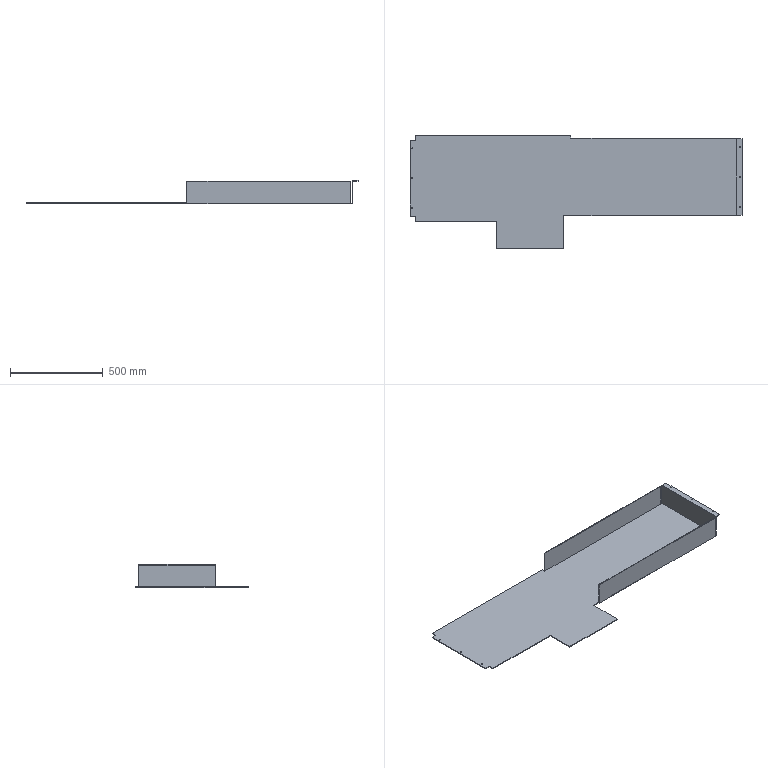Part | STEP file | Guard 8 | 1 solid | 44 faces | box 1787 x 612 x 124 mm | volume 4313397 mm3 | plane 32 | cylinder 12 | commonest cylinder face diameters 6 x12
STEP:
#1=CARTESIAN_POINT('',(16.,199.5,4.));
#2=VERTEX_POINT('',#1);
#3=CARTESIAN_POINT('',(10.,199.5,4.));
#4=VERTEX_POINT('',#3);
#5=CARTESIAN_POINT('',(13.,199.5,4.));
#6=DIRECTION('',(0.,0.,-1.));
#7=DIRECTION('',(-1.,0.,0.));
#8=AXIS2_PLACEMENT_3D('',#5,#6,#7);
#9=CIRCLE('',#8,3.);
#10=EDGE_CURVE('',#2,#4,#9,.T.);
#11=ORIENTED_EDGE('',*,*,#10,.F.);
#12=CARTESIAN_POINT('',(16.,199.5,0.));
#13=VERTEX_POINT('',#12);
#14=CARTESIAN_POINT('',(16.,199.5,10.));
#15=DIRECTION('',(0.,0.,-1.));
#16=VECTOR('',#15,1000.);
#17=LINE('',#14,#16);
#18=EDGE_CURVE('',#2,#13,#17,.T.);
#19=ORIENTED_EDGE('',*,*,#18,.T.);
#20=CARTESIAN_POINT('',(10.,199.5,0.));
#21=VERTEX_POINT('',#20);
#22=CARTESIAN_POINT('',(13.,199.5,0.));
#23=DIRECTION('',(0.,0.,-1.));
#24=DIRECTION('',(-1.,0.,0.));
#25=AXIS2_PLACEMENT_3D('',#22,#23,#24);
#26=CIRCLE('',#25,3.);
#27=EDGE_CURVE('',#13,#21,#26,.T.);
#28=ORIENTED_EDGE('',*,*,#27,.T.);
#29=CARTESIAN_POINT('',(10.,199.5,10.));
#30=DIRECTION('',(0.,0.,-1.));
#31=VECTOR('',#30,1000.);
#32=LINE('',#29,#31);
#33=EDGE_CURVE('',#4,#21,#32,.T.);
#34=ORIENTED_EDGE('',*,*,#33,.F.);
#35=EDGE_LOOP('',(#11,#19,#28,#34));
#36=FACE_OUTER_BOUND('',#35,.T.);
#37=CARTESIAN_POINT('',(13.,199.5,10.));
#38=DIRECTION('',(0.,0.,-1.));
#39=DIRECTION('',(-1.,0.,0.));
#40=AXIS2_PLACEMENT_3D('',#37,#38,#39);
#41=CYLINDRICAL_SURFACE('',#40,3.);
#42=ADVANCED_FACE('',(#36),#41,.F.);
#43=CARTESIAN_POINT('',(16.,39.5,4.));
#44=VERTEX_POINT('',#43);
#45=CARTESIAN_POINT('',(10.,39.5,4.));
#46=VERTEX_POINT('',#45);
#47=CARTESIAN_POINT('',(13.,39.5,4.));
#48=DIRECTION('',(0.,0.,-1.));
#49=DIRECTION('',(-1.,0.,0.));
#50=AXIS2_PLACEMENT_3D('',#47,#48,#49);
#51=CIRCLE('',#50,3.);
#52=EDGE_CURVE('',#44,#46,#51,.T.);
#53=ORIENTED_EDGE('',*,*,#52,.F.);
#54=CARTESIAN_POINT('',(16.,39.5,0.));
#55=VERTEX_POINT('',#54);
#56=CARTESIAN_POINT('',(16.,39.5,10.));
#57=DIRECTION('',(0.,0.,-1.));
#58=VECTOR('',#57,1000.);
#59=LINE('',#56,#58);
#60=EDGE_CURVE('',#44,#55,#59,.T.);
#61=ORIENTED_EDGE('',*,*,#60,.T.);
#62=CARTESIAN_POINT('',(10.,39.5,0.));
#63=VERTEX_POINT('',#62);
#64=CARTESIAN_POINT('',(13.,39.5,0.));
#65=DIRECTION('',(0.,0.,-1.));
#66=DIRECTION('',(-1.,0.,0.));
#67=AXIS2_PLACEMENT_3D('',#64,#65,#66);
#68=CIRCLE('',#67,3.);
#69=EDGE_CURVE('',#55,#63,#68,.T.);
#70=ORIENTED_EDGE('',*,*,#69,.T.);
#71=CARTESIAN_POINT('',(10.,39.5,10.));
#72=DIRECTION('',(0.,0.,-1.));
#73=VECTOR('',#72,1000.);
#74=LINE('',#71,#73);
#75=EDGE_CURVE('',#46,#63,#74,.T.);
#76=ORIENTED_EDGE('',*,*,#75,.F.);
#77=EDGE_LOOP('',(#53,#61,#70,#76));
#78=FACE_OUTER_BOUND('',#77,.T.);
#79=CARTESIAN_POINT('',(13.,39.5,10.));
#80=DIRECTION('',(0.,0.,-1.));
#81=DIRECTION('',(-1.,0.,0.));
#82=AXIS2_PLACEMENT_3D('',#79,#80,#81);
#83=CYLINDRICAL_SURFACE('',#82,3.);
#84=ADVANCED_FACE('',(#78),#83,.F.);
#85=CARTESIAN_POINT('',(16.,359.5,4.));
#86=VERTEX_POINT('',#85);
#87=CARTESIAN_POINT('',(10.,359.5,4.));
#88=VERTEX_POINT('',#87);
#89=CARTESIAN_POINT('',(13.,359.5,4.));
#90=DIRECTION('',(0.,0.,-1.));
#91=DIRECTION('',(-1.,0.,0.));
#92=AXIS2_PLACEMENT_3D('',#89,#90,#91);
#93=CIRCLE('',#92,3.);
#94=EDGE_CURVE('',#86,#88,#93,.T.);
#95=ORIENTED_EDGE('',*,*,#94,.F.);
#96=CARTESIAN_POINT('',(16.,359.5,0.));
#97=VERTEX_POINT('',#96);
#98=CARTESIAN_POINT('',(16.,359.5,10.));
#99=DIRECTION('',(0.,0.,-1.));
#100=VECTOR('',#99,1000.);
#101=LINE('',#98,#100);
#102=EDGE_CURVE('',#86,#97,#101,.T.);
#103=ORIENTED_EDGE('',*,*,#102,.T.);
#104=CARTESIAN_POINT('',(10.,359.5,0.));
#105=VERTEX_POINT('',#104);
#106=CARTESIAN_POINT('',(13.,359.5,0.));
#107=DIRECTION('',(0.,0.,-1.));
#108=DIRECTION('',(-1.,0.,0.));
#109=AXIS2_PLACEMENT_3D('',#106,#107,#108);
#110=CIRCLE('',#109,3.);
#111=EDGE_CURVE('',#97,#105,#110,.T.);
#112=ORIENTED_EDGE('',*,*,#111,.T.);
#113=CARTESIAN_POINT('',(10.,359.5,10.));
#114=DIRECTION('',(0.,0.,-1.));
#115=VECTOR('',#114,1000.);
#116=LINE('',#113,#115);
#117=EDGE_CURVE('',#88,#105,#116,.T.);
#118=ORIENTED_EDGE('',*,*,#117,.F.);
#119=EDGE_LOOP('',(#95,#103,#112,#118));
#120=FACE_OUTER_BOUND('',#119,.T.);
#121=CARTESIAN_POINT('',(13.,359.5,10.));
#122=DIRECTION('',(0.,0.,-1.));
#123=DIRECTION('',(-1.,0.,0.));
#124=AXIS2_PLACEMENT_3D('',#121,#122,#123);
#125=CYLINDRICAL_SURFACE('',#124,3.);
#126=ADVANCED_FACE('',(#120),#125,.F.);
#127=CARTESIAN_POINT('',(1774.,205.5,124.));
#128=VERTEX_POINT('',#127);
#129=CARTESIAN_POINT('',(1780.,205.5,124.));
#130=VERTEX_POINT('',#129);
#131=CARTESIAN_POINT('',(1777.,205.5,124.));
#132=DIRECTION('',(0.,0.,1.));
#133=DIRECTION('',(1.,0.,0.));
#134=AXIS2_PLACEMENT_3D('',#131,#132,#133);
#135=CIRCLE('',#134,3.);
#136=EDGE_CURVE('',#128,#130,#135,.T.);
#137=ORIENTED_EDGE('',*,*,#136,.T.);
#138=CARTESIAN_POINT('',(1780.,205.5,121.));
#139=VERTEX_POINT('',#138);
#140=CARTESIAN_POINT('',(1780.,205.5,131.));
#141=DIRECTION('',(0.,0.,-1.));
#142=VECTOR('',#141,1000.);
#143=LINE('',#140,#142);
#144=EDGE_CURVE('',#130,#139,#143,.T.);
#145=ORIENTED_EDGE('',*,*,#144,.T.);
#146=CARTESIAN_POINT('',(1774.,205.5,121.));
#147=VERTEX_POINT('',#146);
#148=CARTESIAN_POINT('',(1777.,205.5,121.));
#149=DIRECTION('',(0.,0.,-1.));
#150=DIRECTION('',(-1.,0.,0.));
#151=AXIS2_PLACEMENT_3D('',#148,#149,#150);
#152=CIRCLE('',#151,3.);
#153=EDGE_CURVE('',#139,#147,#152,.T.);
#154=ORIENTED_EDGE('',*,*,#153,.T.);
#155=CARTESIAN_POINT('',(1774.,205.5,131.));
#156=DIRECTION('',(0.,0.,-1.));
#157=VECTOR('',#156,1000.);
#158=LINE('',#155,#157);
#159=EDGE_CURVE('',#128,#147,#158,.T.);
#160=ORIENTED_EDGE('',*,*,#159,.F.);
#161=EDGE_LOOP('',(#137,#145,#154,#160));
#162=FACE_OUTER_BOUND('',#161,.T.);
#163=CARTESIAN_POINT('',(1777.,205.5,131.));
#164=DIRECTION('',(0.,0.,-1.));
#165=DIRECTION('',(-1.,0.,0.));
#166=AXIS2_PLACEMENT_3D('',#163,#164,#165);
#167=CYLINDRICAL_SURFACE('',#166,3.);
#168=ADVANCED_FACE('',(#162),#167,.F.);
#169=CARTESIAN_POINT('',(1774.,45.5,124.));
#170=VERTEX_POINT('',#169);
#171=CARTESIAN_POINT('',(1780.,45.5,124.));
#172=VERTEX_POINT('',#171);
#173=CARTESIAN_POINT('',(1777.,45.5,124.));
#174=DIRECTION('',(0.,0.,1.));
#175=DIRECTION('',(1.,0.,0.));
#176=AXIS2_PLACEMENT_3D('',#173,#174,#175);
#177=CIRCLE('',#176,3.);
#178=EDGE_CURVE('',#170,#172,#177,.T.);
#179=ORIENTED_EDGE('',*,*,#178,.T.);
#180=CARTESIAN_POINT('',(1780.,45.5,121.));
#181=VERTEX_POINT('',#180);
#182=CARTESIAN_POINT('',(1780.,45.5,131.));
#183=DIRECTION('',(0.,0.,-1.));
#184=VECTOR('',#183,1000.);
#185=LINE('',#182,#184);
#186=EDGE_CURVE('',#172,#181,#185,.T.);
#187=ORIENTED_EDGE('',*,*,#186,.T.);
#188=CARTESIAN_POINT('',(1774.,45.5,121.));
#189=VERTEX_POINT('',#188);
#190=CARTESIAN_POINT('',(1777.,45.5,121.));
#191=DIRECTION('',(0.,0.,-1.));
#192=DIRECTION('',(-1.,0.,0.));
#193=AXIS2_PLACEMENT_3D('',#190,#191,#192);
#194=CIRCLE('',#193,3.);
#195=EDGE_CURVE('',#181,#189,#194,.T.);
#196=ORIENTED_EDGE('',*,*,#195,.T.);
#197=CARTESIAN_POINT('',(1774.,45.5,131.));
#198=DIRECTION('',(0.,0.,-1.));
#199=VECTOR('',#198,1000.);
#200=LINE('',#197,#199);
#201=EDGE_CURVE('',#170,#189,#200,.T.);
#202=ORIENTED_EDGE('',*,*,#201,.F.);
#203=EDGE_LOOP('',(#179,#187,#196,#202));
#204=FACE_OUTER_BOUND('',#203,.T.);
#205=CARTESIAN_POINT('',(1777.,45.5,131.));
#206=DIRECTION('',(0.,0.,-1.));
#207=DIRECTION('',(-1.,0.,0.));
#208=AXIS2_PLACEMENT_3D('',#205,#206,#207);
#209=CYLINDRICAL_SURFACE('',#208,3.);
#210=ADVANCED_FACE('',(#204),#209,.F.);
#211=CARTESIAN_POINT('',(1774.,365.5,124.));
#212=VERTEX_POINT('',#211);
#213=CARTESIAN_POINT('',(1780.,365.5,124.));
#214=VERTEX_POINT('',#213);
#215=CARTESIAN_POINT('',(1777.,365.5,124.));
#216=DIRECTION('',(0.,0.,1.));
#217=DIRECTION('',(1.,0.,0.));
#218=AXIS2_PLACEMENT_3D('',#215,#216,#217);
#219=CIRCLE('',#218,3.);
#220=EDGE_CURVE('',#212,#214,#219,.T.);
#221=ORIENTED_EDGE('',*,*,#220,.T.);
#222=CARTESIAN_POINT('',(1780.,365.5,121.));
#223=VERTEX_POINT('',#222);
#224=CARTESIAN_POINT('',(1780.,365.5,131.));
#225=DIRECTION('',(0.,0.,-1.));
#226=VECTOR('',#225,1000.);
#227=LINE('',#224,#226);
#228=EDGE_CURVE('',#214,#223,#227,.T.);
#229=ORIENTED_EDGE('',*,*,#228,.T.);
#230=CARTESIAN_POINT('',(1774.,365.5,121.));
#231=VERTEX_POINT('',#230);
#232=CARTESIAN_POINT('',(1777.,365.5,121.));
#233=DIRECTION('',(0.,0.,-1.));
#234=DIRECTION('',(-1.,0.,0.));
#235=AXIS2_PLACEMENT_3D('',#232,#233,#234);
#236=CIRCLE('',#235,3.);
#237=EDGE_CURVE('',#223,#231,#236,.T.);
#238=ORIENTED_EDGE('',*,*,#237,.T.);
#239=CARTESIAN_POINT('',(1774.,365.5,131.));
#240=DIRECTION('',(0.,0.,-1.));
#241=VECTOR('',#240,1000.);
#242=LINE('',#239,#241);
#243=EDGE_CURVE('',#212,#231,#242,.T.);
#244=ORIENTED_EDGE('',*,*,#243,.F.);
#245=EDGE_LOOP('',(#221,#229,#238,#244));
#246=FACE_OUTER_BOUND('',#245,.T.);
#247=CARTESIAN_POINT('',(1777.,365.5,131.));
#248=DIRECTION('',(0.,0.,-1.));
#249=DIRECTION('',(-1.,0.,0.));
#250=AXIS2_PLACEMENT_3D('',#247,#248,#249);
#251=CYLINDRICAL_SURFACE('',#250,3.);
#252=ADVANCED_FACE('',(#246),#251,.F.);
#253=CARTESIAN_POINT('',(866.,415.,4.));
#254=VERTEX_POINT('',#253);
#255=CARTESIAN_POINT('',(866.,411.,4.));
#256=VERTEX_POINT('',#255);
#257=CARTESIAN_POINT('',(866.,431.,4.));
#258=DIRECTION('',(0.,-1.,0.));
#259=VECTOR('',#258,1000.);
#260=LINE('',#257,#259);
#261=EDGE_CURVE('',#254,#256,#260,.T.);
#262=ORIENTED_EDGE('',*,*,#261,.T.);
#263=CARTESIAN_POINT('',(866.,411.,121.));
#264=VERTEX_POINT('',#263);
#265=CARTESIAN_POINT('',(866.,411.,0.));
#266=DIRECTION('',(0.,0.,-1.));
#267=VECTOR('',#266,1000.);
#268=LINE('',#265,#267);
#269=EDGE_CURVE('',#264,#256,#268,.T.);
#270=ORIENTED_EDGE('',*,*,#269,.F.);
#271=CARTESIAN_POINT('',(866.,415.,121.));
#272=VERTEX_POINT('',#271);
#273=CARTESIAN_POINT('',(866.,411.,121.));
#274=DIRECTION('',(0.,1.,0.));
#275=VECTOR('',#274,1000.);
#276=LINE('',#273,#275);
#277=EDGE_CURVE('',#264,#272,#276,.T.);
#278=ORIENTED_EDGE('',*,*,#277,.T.);
#279=CARTESIAN_POINT('',(866.,415.,0.));
#280=DIRECTION('',(0.,0.,-1.));
#281=VECTOR('',#280,1000.);
#282=LINE('',#279,#281);
#283=EDGE_CURVE('',#272,#254,#282,.T.);
#284=ORIENTED_EDGE('',*,*,#283,.T.);
#285=EDGE_LOOP('',(#262,#270,#278,#284));
#286=FACE_OUTER_BOUND('',#285,.T.);
#287=CARTESIAN_POINT('',(866.,411.,0.));
#288=DIRECTION('',(1.,0.,0.));
#289=DIRECTION('',(0.,0.,-1.));
#290=AXIS2_PLACEMENT_3D('',#287,#288,#289);
#291=PLANE('',#290);
#292=ADVANCED_FACE('',(#286),#291,.F.);
#293=CARTESIAN_POINT('',(1760.,411.,0.));
#294=VERTEX_POINT('',#293);
#295=CARTESIAN_POINT('',(1748.,411.,0.));
#296=VERTEX_POINT('',#295);
#297=CARTESIAN_POINT('',(0.,411.,0.));
#298=DIRECTION('',(-1.,0.,0.));
#299=VECTOR('',#298,1000.);
#300=LINE('',#297,#299);
#301=EDGE_CURVE('',#294,#296,#300,.T.);
#302=ORIENTED_EDGE('',*,*,#301,.T.);
#303=CARTESIAN_POINT('',(1748.,411.,4.));
#304=VERTEX_POINT('',#303);
#305=CARTESIAN_POINT('',(1748.,411.,0.));
#306=DIRECTION('',(0.,0.,1.));
#307=VECTOR('',#306,1000.);
#308=LINE('',#305,#307);
#309=EDGE_CURVE('',#296,#304,#308,.T.);
#310=ORIENTED_EDGE('',*,*,#309,.T.);
#311=CARTESIAN_POINT('',(1757.,411.,4.));
#312=VERTEX_POINT('',#311);
#313=CARTESIAN_POINT('',(0.,411.,4.));
#314=DIRECTION('',(-1.,0.,0.));
#315=VECTOR('',#314,1000.);
#316=LINE('',#313,#315);
#317=EDGE_CURVE('',#312,#304,#316,.T.);
#318=ORIENTED_EDGE('',*,*,#317,.F.);
#319=CARTESIAN_POINT('',(1757.,411.,124.));
#320=VERTEX_POINT('',#319);
#321=CARTESIAN_POINT('',(1757.,411.,4.));
#322=DIRECTION('',(0.,0.,-1.));
#323=VECTOR('',#322,1000.);
#324=LINE('',#321,#323);
#325=EDGE_CURVE('',#320,#312,#324,.T.);
#326=ORIENTED_EDGE('',*,*,#325,.F.);
#327=CARTESIAN_POINT('',(1787.,411.,124.));
#328=VERTEX_POINT('',#327);
#329=CARTESIAN_POINT('',(1760.,411.,124.));
#330=DIRECTION('',(-1.,0.,0.));
#331=VECTOR('',#330,1000.);
#332=LINE('',#329,#331);
#333=EDGE_CURVE('',#328,#320,#332,.T.);
#334=ORIENTED_EDGE('',*,*,#333,.F.);
#335=CARTESIAN_POINT('',(1787.,411.,121.));
#336=VERTEX_POINT('',#335);
#337=CARTESIAN_POINT('',(1787.,411.,124.));
#338=DIRECTION('',(0.,0.,1.));
#339=VECTOR('',#338,1000.);
#340=LINE('',#337,#339);
#341=EDGE_CURVE('',#336,#328,#340,.T.);
#342=ORIENTED_EDGE('',*,*,#341,.F.);
#343=CARTESIAN_POINT('',(1760.,411.,121.));
#344=VERTEX_POINT('',#343);
#345=CARTESIAN_POINT('',(1787.,411.,121.));
#346=DIRECTION('',(1.,0.,0.));
#347=VECTOR('',#346,1000.);
#348=LINE('',#345,#347);
#349=EDGE_CURVE('',#344,#336,#348,.T.);
#350=ORIENTED_EDGE('',*,*,#349,.F.);
#351=CARTESIAN_POINT('',(1760.,411.,0.));
#352=DIRECTION('',(0.,0.,1.));
#353=VECTOR('',#352,1000.);
#354=LINE('',#351,#353);
#355=EDGE_CURVE('',#294,#344,#354,.T.);
#356=ORIENTED_EDGE('',*,*,#355,.F.);
#357=EDGE_LOOP('',(#302,#310,#318,#326,#334,#342,#350,#356));
#358=FACE_OUTER_BOUND('',#357,.T.);
#359=CARTESIAN_POINT('',(0.,411.,4.));
#360=DIRECTION('',(0.,-1.,0.));
#361=DIRECTION('',(0.,0.,-1.));
#362=AXIS2_PLACEMENT_3D('',#359,#360,#361);
#363=PLANE('',#362);
#364=ADVANCED_FACE('',(#358),#363,.F.);
#365=CARTESIAN_POINT('',(1748.,0.,0.));
#366=VERTEX_POINT('',#365);
#367=CARTESIAN_POINT('',(1748.,0.,4.));
#368=VERTEX_POINT('',#367);
#369=CARTESIAN_POINT('',(1748.,0.,0.));
#370=DIRECTION('',(0.,0.,1.));
#371=VECTOR('',#370,1000.);
#372=LINE('',#369,#371);
#373=EDGE_CURVE('',#366,#368,#372,.T.);
#374=ORIENTED_EDGE('',*,*,#373,.F.);
#375=CARTESIAN_POINT('',(1760.,0.,0.));
#376=VERTEX_POINT('',#375);
#377=CARTESIAN_POINT('',(0.,0.,0.));
#378=DIRECTION('',(1.,0.,0.));
#379=VECTOR('',#378,1000.);
#380=LINE('',#377,#379);
#381=EDGE_CURVE('',#366,#376,#380,.T.);
#382=ORIENTED_EDGE('',*,*,#381,.T.);
#383=CARTESIAN_POINT('',(1760.,0.,121.));
#384=VERTEX_POINT('',#383);
#385=CARTESIAN_POINT('',(1760.,0.,4.));
#386=DIRECTION('',(0.,0.,-1.));
#387=VECTOR('',#386,1000.);
#388=LINE('',#385,#387);
#389=EDGE_CURVE('',#384,#376,#388,.T.);
#390=ORIENTED_EDGE('',*,*,#389,.F.);
#391=CARTESIAN_POINT('',(1787.,0.,121.));
#392=VERTEX_POINT('',#391);
#393=CARTESIAN_POINT('',(1787.,0.,121.));
#394=DIRECTION('',(1.,0.,0.));
#395=VECTOR('',#394,1000.);
#396=LINE('',#393,#395);
#397=EDGE_CURVE('',#384,#392,#396,.T.);
#398=ORIENTED_EDGE('',*,*,#397,.T.);
#399=CARTESIAN_POINT('',(1787.,0.,124.));
#400=VERTEX_POINT('',#399);
#401=CARTESIAN_POINT('',(1787.,0.,124.));
#402=DIRECTION('',(0.,0.,1.));
#403=VECTOR('',#402,1000.);
#404=LINE('',#401,#403);
#405=EDGE_CURVE('',#392,#400,#404,.T.);
#406=ORIENTED_EDGE('',*,*,#405,.T.);
#407=CARTESIAN_POINT('',(1757.,0.,124.));
#408=VERTEX_POINT('',#407);
#409=CARTESIAN_POINT('',(1760.,0.,124.));
#410=DIRECTION('',(-1.,0.,0.));
#411=VECTOR('',#410,1000.);
#412=LINE('',#409,#411);
#413=EDGE_CURVE('',#400,#408,#412,.T.);
#414=ORIENTED_EDGE('',*,*,#413,.T.);
#415=CARTESIAN_POINT('',(1757.,0.,4.));
#416=VERTEX_POINT('',#415);
#417=CARTESIAN_POINT('',(1757.,0.,4.));
#418=DIRECTION('',(0.,0.,-1.));
#419=VECTOR('',#418,1000.);
#420=LINE('',#417,#419);
#421=EDGE_CURVE('',#408,#416,#420,.T.);
#422=ORIENTED_EDGE('',*,*,#421,.T.);
#423=CARTESIAN_POINT('',(0.,0.,4.));
#424=DIRECTION('',(1.,0.,0.));
#425=VECTOR('',#424,1000.);
#426=LINE('',#423,#425);
#427=EDGE_CURVE('',#368,#416,#426,.T.);
#428=ORIENTED_EDGE('',*,*,#427,.F.);
#429=EDGE_LOOP('',(#374,#382,#390,#398,#406,#414,#422,#428));
#430=FACE_OUTER_BOUND('',#429,.T.);
#431=CARTESIAN_POINT('',(0.,0.,4.));
#432=DIRECTION('',(0.,1.,0.));
#433=DIRECTION('',(0.,0.,1.));
#434=AXIS2_PLACEMENT_3D('',#431,#432,#433);
#435=PLANE('',#434);
#436=ADVANCED_FACE('',(#430),#435,.F.);
#437=CARTESIAN_POINT('',(866.,0.,4.));
#438=VERTEX_POINT('',#437);
#439=CARTESIAN_POINT('',(866.,0.,0.));
#440=VERTEX_POINT('',#439);
#441=CARTESIAN_POINT('',(866.,0.,0.));
#442=DIRECTION('',(0.,0.,-1.));
#443=VECTOR('',#442,1000.);
#444=LINE('',#441,#443);
#445=EDGE_CURVE('',#438,#440,#444,.T.);
#446=ORIENTED_EDGE('',*,*,#445,.F.);
#447=CARTESIAN_POINT('',(826.,0.,4.));
#448=VERTEX_POINT('',#447);
#449=CARTESIAN_POINT('',(0.,0.,4.));
#450=DIRECTION('',(1.,0.,0.));
#451=VECTOR('',#450,1000.);
#452=LINE('',#449,#451);
#453=EDGE_CURVE('',#448,#438,#452,.T.);
#454=ORIENTED_EDGE('',*,*,#453,.F.);
#455=CARTESIAN_POINT('',(826.,0.,0.));
#456=VERTEX_POINT('',#455);
#457=CARTESIAN_POINT('',(826.,0.,0.));
#458=DIRECTION('',(0.,0.,1.));
#459=VECTOR('',#458,1000.);
#460=LINE('',#457,#459);
#461=EDGE_CURVE('',#456,#448,#460,.T.);
#462=ORIENTED_EDGE('',*,*,#461,.F.);
#463=CARTESIAN_POINT('',(0.,0.,0.));
#464=DIRECTION('',(1.,0.,0.));
#465=VECTOR('',#464,1000.);
#466=LINE('',#463,#465);
#467=EDGE_CURVE('',#456,#440,#466,.T.);
#468=ORIENTED_EDGE('',*,*,#467,.T.);
#469=EDGE_LOOP('',(#446,#454,#462,#468));
#470=FACE_OUTER_BOUND('',#469,.T.);
#471=CARTESIAN_POINT('',(0.,0.,4.));
#472=DIRECTION('',(0.,1.,0.));
#473=DIRECTION('',(0.,0.,1.));
#474=AXIS2_PLACEMENT_3D('',#471,#472,#473);
#475=PLANE('',#474);
#476=ADVANCED_FACE('',(#470),#475,.F.);
#477=CARTESIAN_POINT('',(13.,199.5,4.));
#478=DIRECTION('',(0.,0.,-1.));
#479=DIRECTION('',(-1.,0.,0.));
#480=AXIS2_PLACEMENT_3D('',#477,#478,#479);
#481=CIRCLE('',#480,3.);
#482=EDGE_CURVE('',#4,#2,#481,.T.);
#483=ORIENTED_EDGE('',*,*,#482,.T.);
#484=ORIENTED_EDGE('',*,*,#10,.T.);
#485=EDGE_LOOP('',(#483,#484));
#486=FACE_BOUND('',#485,.T.);
#487=CARTESIAN_POINT('',(13.,39.5,4.));
#488=DIRECTION('',(0.,0.,-1.));
#489=DIRECTION('',(-1.,0.,0.));
#490=AXIS2_PLACEMENT_3D('',#487,#488,#489);
#491=CIRCLE('',#490,3.);
#492=EDGE_CURVE('',#46,#44,#491,.T.);
#493=ORIENTED_EDGE('',*,*,#492,.T.);
#494=ORIENTED_EDGE('',*,*,#52,.T.);
#495=EDGE_LOOP('',(#493,#494));
#496=FACE_BOUND('',#495,.T.);
#497=CARTESIAN_POINT('',(13.,359.5,4.));
#498=DIRECTION('',(0.,0.,-1.));
#499=DIRECTION('',(-1.,0.,0.));
#500=AXIS2_PLACEMENT_3D('',#497,#498,#499);
#501=CIRCLE('',#500,3.);
#502=EDGE_CURVE('',#88,#86,#501,.T.);
#503=ORIENTED_EDGE('',*,*,#502,.T.);
#504=ORIENTED_EDGE('',*,*,#94,.T.);
#505=EDGE_LOOP('',(#503,#504));
#506=FACE_BOUND('',#505,.T.);
#507=CARTESIAN_POINT('',(0.,404.,4.));
#508=VERTEX_POINT('',#507);
#509=CARTESIAN_POINT('',(0.,-5.,4.));
#510=VERTEX_POINT('',#509);
#511=CARTESIAN_POINT('',(0.,0.,4.));
#512=DIRECTION('',(0.,-1.,0.));
#513=VECTOR('',#512,1000.);
#514=LINE('',#511,#513);
#515=EDGE_CURVE('',#508,#510,#514,.T.);
#516=ORIENTED_EDGE('',*,*,#515,.T.);
#517=CARTESIAN_POINT('',(27.,-5.,4.));
#518=VERTEX_POINT('',#517);
#519=CARTESIAN_POINT('',(0.,-5.,4.));
#520=DIRECTION('',(-1.,0.,0.));
#521=VECTOR('',#520,1000.);
#522=LINE('',#519,#521);
#523=EDGE_CURVE('',#518,#510,#522,.T.);
#524=ORIENTED_EDGE('',*,*,#523,.F.);
#525=CARTESIAN_POINT('',(27.,-32.,4.));
#526=VERTEX_POINT('',#525);
#527=CARTESIAN_POINT('',(27.,-32.,4.));
#528=DIRECTION('',(0.,1.,0.));
#529=VECTOR('',#528,1000.);
#530=LINE('',#527,#529);
#531=EDGE_CURVE('',#526,#518,#530,.T.);
#532=ORIENTED_EDGE('',*,*,#531,.F.);
#533=CARTESIAN_POINT('',(463.,-32.,4.));
#534=VERTEX_POINT('',#533);
#535=CARTESIAN_POINT('',(463.,-32.,4.));
#536=DIRECTION('',(-1.,0.,0.));
#537=VECTOR('',#536,1000.);
#538=LINE('',#535,#537);
#539=EDGE_CURVE('',#534,#526,#538,.T.);
#540=ORIENTED_EDGE('',*,*,#539,.F.);
#541=CARTESIAN_POINT('',(463.,-181.,4.));
#542=VERTEX_POINT('',#541);
#543=CARTESIAN_POINT('',(463.,0.,4.));
#544=DIRECTION('',(0.,-1.,0.));
#545=VECTOR('',#544,1000.);
#546=LINE('',#543,#545);
#547=EDGE_CURVE('',#534,#542,#546,.T.);
#548=ORIENTED_EDGE('',*,*,#547,.T.);
#549=CARTESIAN_POINT('',(826.,-181.,4.));
#550=VERTEX_POINT('',#549);
#551=CARTESIAN_POINT('',(463.,-181.,4.));
#552=DIRECTION('',(1.,0.,0.));
#553=VECTOR('',#552,1000.);
#554=LINE('',#551,#553);
#555=EDGE_CURVE('',#542,#550,#554,.T.);
#556=ORIENTED_EDGE('',*,*,#555,.T.);
#557=CARTESIAN_POINT('',(826.,0.,4.));
#558=DIRECTION('',(0.,1.,0.));
#559=VECTOR('',#558,1000.);
#560=LINE('',#557,#559);
#561=EDGE_CURVE('',#550,#448,#560,.T.);
#562=ORIENTED_EDGE('',*,*,#561,.T.);
#563=ORIENTED_EDGE('',*,*,#453,.T.);
#564=CARTESIAN_POINT('',(866.,-4.,4.));
#565=VERTEX_POINT('',#564);
#566=CARTESIAN_POINT('',(866.,-4.,4.));
#567=DIRECTION('',(0.,1.,0.));
#568=VECTOR('',#567,1000.);
#569=LINE('',#566,#568);
#570=EDGE_CURVE('',#565,#438,#569,.T.);
#571=ORIENTED_EDGE('',*,*,#570,.F.);
#572=CARTESIAN_POINT('',(866.,-4.,4.));
#573=VERTEX_POINT('',#572);
#574=CARTESIAN_POINT('',(1748.,-4.,4.));
#575=DIRECTION('',(-1.,0.,0.));
#576=VECTOR('',#575,1000.);
#577=LINE('',#574,#576);
#578=EDGE_CURVE('',#573,#565,#577,.T.);
#579=ORIENTED_EDGE('',*,*,#578,.F.);
#580=CARTESIAN_POINT('',(866.,0.,4.));
#581=VERTEX_POINT('',#580);
#582=CARTESIAN_POINT('',(866.,0.,4.));
#583=DIRECTION('',(0.,1.,0.));
#584=VECTOR('',#583,1000.);
#585=LINE('',#582,#584);
#586=EDGE_CURVE('',#573,#581,#585,.T.);
#587=ORIENTED_EDGE('',*,*,#586,.T.);
#588=CARTESIAN_POINT('',(0.,0.,4.));
#589=DIRECTION('',(-1.,0.,0.));
#590=VECTOR('',#589,1000.);
#591=LINE('',#588,#590);
#592=EDGE_CURVE('',#368,#581,#591,.T.);
#593=ORIENTED_EDGE('',*,*,#592,.F.);
#594=ORIENTED_EDGE('',*,*,#427,.T.);
#595=CARTESIAN_POINT('',(1757.,411.,4.));
#596=DIRECTION('',(0.,-1.,0.));
#597=VECTOR('',#596,1000.);
#598=LINE('',#595,#597);
#599=EDGE_CURVE('',#312,#416,#598,.T.);
#600=ORIENTED_EDGE('',*,*,#599,.F.);
#601=ORIENTED_EDGE('',*,*,#317,.T.);
#602=CARTESIAN_POINT('',(0.,411.,4.));
#603=DIRECTION('',(-1.,0.,0.));
#604=VECTOR('',#603,1000.);
#605=LINE('',#602,#604);
#606=EDGE_CURVE('',#304,#256,#605,.T.);
#607=ORIENTED_EDGE('',*,*,#606,.T.);
#608=ORIENTED_EDGE('',*,*,#261,.F.);
#609=CARTESIAN_POINT('',(866.,431.,4.));
#610=VERTEX_POINT('',#609);
#611=CARTESIAN_POINT('',(866.,431.,4.));
#612=DIRECTION('',(0.,-1.,0.));
#613=VECTOR('',#612,1000.);
#614=LINE('',#611,#613);
#615=EDGE_CURVE('',#610,#254,#614,.T.);
#616=ORIENTED_EDGE('',*,*,#615,.F.);
#617=CARTESIAN_POINT('',(27.,431.,4.));
#618=VERTEX_POINT('',#617);
#619=CARTESIAN_POINT('',(0.,431.,4.));
#620=DIRECTION('',(1.,0.,0.));
#621=VECTOR('',#620,1000.);
#622=LINE('',#619,#621);
#623=EDGE_CURVE('',#618,#610,#622,.T.);
#624=ORIENTED_EDGE('',*,*,#623,.F.);
#625=CARTESIAN_POINT('',(27.,404.,4.));
#626=VERTEX_POINT('',#625);
#627=CARTESIAN_POINT('',(27.,431.,4.));
#628=DIRECTION('',(0.,1.,0.));
#629=VECTOR('',#628,1000.);
#630=LINE('',#627,#629);
#631=EDGE_CURVE('',#626,#618,#630,.T.);
#632=ORIENTED_EDGE('',*,*,#631,.F.);
#633=CARTESIAN_POINT('',(0.,404.,4.));
#634=DIRECTION('',(1.,0.,0.));
#635=VECTOR('',#634,1000.);
#636=LINE('',#633,#635);
#637=EDGE_CURVE('',#508,#626,#636,.T.);
#638=ORIENTED_EDGE('',*,*,#637,.F.);
#639=EDGE_LOOP('',(#516,#524,#532,#540,#548,#556,#562,#563,#571,#579,#587,#593,#594,#600,#601,#607,#608,#616,#624,#632,#638));
#640=FACE_OUTER_BOUND('',#639,.T.);
#641=CARTESIAN_POINT('',(0.,0.,4.));
#642=DIRECTION('',(0.,0.,-1.));
#643=DIRECTION('',(-1.,0.,0.));
#644=AXIS2_PLACEMENT_3D('',#641,#642,#643);
#645=PLANE('',#644);
#646=ADVANCED_FACE('',(#486,#496,#506,#640),#645,.F.);
#647=CARTESIAN_POINT('',(0.,404.,0.));
#648=VERTEX_POINT('',#647);
#649=CARTESIAN_POINT('',(0.,-5.,0.));
#650=VERTEX_POINT('',#649);
#651=CARTESIAN_POINT('',(0.,0.,0.));
#652=DIRECTION('',(0.,-1.,0.));
#653=VECTOR('',#652,1000.);
#654=LINE('',#651,#653);
#655=EDGE_CURVE('',#648,#650,#654,.T.);
#656=ORIENTED_EDGE('',*,*,#655,.T.);
#657=CARTESIAN_POINT('',(0.,-5.,-27.));
#658=DIRECTION('',(0.,0.,1.));
#659=VECTOR('',#658,1000.);
#660=LINE('',#657,#659);
#661=EDGE_CURVE('',#650,#510,#660,.T.);
#662=ORIENTED_EDGE('',*,*,#661,.T.);
#663=ORIENTED_EDGE('',*,*,#515,.F.);
#664=CARTESIAN_POINT('',(0.,404.,-27.));
#665=DIRECTION('',(0.,0.,1.));
#666=VECTOR('',#665,1000.);
#667=LINE('',#664,#666);
#668=EDGE_CURVE('',#648,#508,#667,.T.);
#669=ORIENTED_EDGE('',*,*,#668,.F.);
#670=EDGE_LOOP('',(#656,#662,#663,#669));
#671=FACE_OUTER_BOUND('',#670,.T.);
#672=CARTESIAN_POINT('',(0.,0.,4.));
#673=DIRECTION('',(1.,0.,0.));
#674=DIRECTION('',(0.,0.,-1.));
#675=AXIS2_PLACEMENT_3D('',#672,#673,#674);
#676=PLANE('',#675);
#677=ADVANCED_FACE('',(#671),#676,.F.);
#678=CARTESIAN_POINT('',(13.,199.5,0.));
#679=DIRECTION('',(0.,0.,-1.));
#680=DIRECTION('',(-1.,0.,0.));
#681=AXIS2_PLACEMENT_3D('',#678,#679,#680);
#682=CIRCLE('',#681,3.);
#683=EDGE_CURVE('',#21,#13,#682,.T.);
#684=ORIENTED_EDGE('',*,*,#683,.F.);
#685=ORIENTED_EDGE('',*,*,#27,.F.);
#686=EDGE_LOOP('',(#684,#685));
#687=FACE_BOUND('',#686,.T.);
#688=CARTESIAN_POINT('',(13.,39.5,0.));
#689=DIRECTION('',(0.,0.,-1.));
#690=DIRECTION('',(-1.,0.,0.));
#691=AXIS2_PLACEMENT_3D('',#688,#689,#690);
#692=CIRCLE('',#691,3.);
#693=EDGE_CURVE('',#63,#55,#692,.T.);
#694=ORIENTED_EDGE('',*,*,#693,.F.);
#695=ORIENTED_EDGE('',*,*,#69,.F.);
#696=EDGE_LOOP('',(#694,#695));
#697=FACE_BOUND('',#696,.T.);
#698=CARTESIAN_POINT('',(13.,359.5,0.));
#699=DIRECTION('',(0.,0.,-1.));
#700=DIRECTION('',(-1.,0.,0.));
#701=AXIS2_PLACEMENT_3D('',#698,#699,#700);
#702=CIRCLE('',#701,3.);
#703=EDGE_CURVE('',#105,#97,#702,.T.);
#704=ORIENTED_EDGE('',*,*,#703,.F.);
#705=ORIENTED_EDGE('',*,*,#111,.F.);
#706=EDGE_LOOP('',(#704,#705));
#707=FACE_BOUND('',#706,.T.);
#708=CARTESIAN_POINT('',(27.,-5.,0.));
#709=VERTEX_POINT('',#708);
#710=CARTESIAN_POINT('',(0.,-5.,0.));
#711=DIRECTION('',(1.,0.,0.));
#712=VECTOR('',#711,1000.);
#713=LINE('',#710,#712);
#714=EDGE_CURVE('',#650,#709,#713,.T.);
#715=ORIENTED_EDGE('',*,*,#714,.F.);
#716=ORIENTED_EDGE('',*,*,#655,.F.);
#717=CARTESIAN_POINT('',(27.,404.,0.));
#718=VERTEX_POINT('',#717);
#719=CARTESIAN_POINT('',(0.,404.,0.));
#720=DIRECTION('',(-1.,0.,0.));
#721=VECTOR('',#720,1000.);
#722=LINE('',#719,#721);
#723=EDGE_CURVE('',#718,#648,#722,.T.);
#724=ORIENTED_EDGE('',*,*,#723,.F.);
#725=CARTESIAN_POINT('',(27.,431.,0.));
#726=VERTEX_POINT('',#725);
#727=CARTESIAN_POINT('',(27.,0.,0.));
#728=DIRECTION('',(0.,-1.,0.));
#729=VECTOR('',#728,1000.);
#730=LINE('',#727,#729);
#731=EDGE_CURVE('',#726,#718,#730,.T.);
#732=ORIENTED_EDGE('',*,*,#731,.F.);
#733=CARTESIAN_POINT('',(866.,431.,0.));
#734=VERTEX_POINT('',#733);
#735=CARTESIAN_POINT('',(866.,431.,0.));
#736=DIRECTION('',(-1.,0.,0.));
#737=VECTOR('',#736,1000.);
#738=LINE('',#735,#737);
#739=EDGE_CURVE('',#734,#726,#738,.T.);
#740=ORIENTED_EDGE('',*,*,#739,.F.);
#741=CARTESIAN_POINT('',(866.,415.,0.));
#742=VERTEX_POINT('',#741);
#743=CARTESIAN_POINT('',(866.,431.,0.));
#744=DIRECTION('',(0.,-1.,0.));
#745=VECTOR('',#744,1000.);
#746=LINE('',#743,#745);
#747=EDGE_CURVE('',#734,#742,#746,.T.);
#748=ORIENTED_EDGE('',*,*,#747,.T.);
#749=CARTESIAN_POINT('',(1748.,415.,0.));
#750=VERTEX_POINT('',#749);
#751=CARTESIAN_POINT('',(1748.,415.,0.));
#752=DIRECTION('',(1.,0.,0.));
#753=VECTOR('',#752,1000.);
#754=LINE('',#751,#753);
#755=EDGE_CURVE('',#742,#750,#754,.T.);
#756=ORIENTED_EDGE('',*,*,#755,.T.);
#757=CARTESIAN_POINT('',(1748.,411.,0.));
#758=DIRECTION('',(0.,1.,0.));
#759=VECTOR('',#758,1000.);
#760=LINE('',#757,#759);
#761=EDGE_CURVE('',#296,#750,#760,.T.);
#762=ORIENTED_EDGE('',*,*,#761,.F.);
#763=ORIENTED_EDGE('',*,*,#301,.F.);
#764=CARTESIAN_POINT('',(1760.,0.,0.));
#765=DIRECTION('',(0.,1.,0.));
#766=VECTOR('',#765,1000.);
#767=LINE('',#764,#766);
#768=EDGE_CURVE('',#376,#294,#767,.T.);
#769=ORIENTED_EDGE('',*,*,#768,.F.);
#770=ORIENTED_EDGE('',*,*,#381,.F.);
#771=CARTESIAN_POINT('',(1748.,-4.,0.));
#772=VERTEX_POINT('',#771);
#773=CARTESIAN_POINT('',(1748.,-4.,0.));
#774=DIRECTION('',(0.,1.,0.));
#775=VECTOR('',#774,1000.);
#776=LINE('',#773,#775);
#777=EDGE_CURVE('',#772,#366,#776,.T.);
#778=ORIENTED_EDGE('',*,*,#777,.F.);
#779=CARTESIAN_POINT('',(866.,-4.,0.));
#780=VERTEX_POINT('',#779);
#781=CARTESIAN_POINT('',(1748.,-4.,0.));
#782=DIRECTION('',(1.,0.,0.));
#783=VECTOR('',#782,1000.);
#784=LINE('',#781,#783);
#785=EDGE_CURVE('',#780,#772,#784,.T.);
#786=ORIENTED_EDGE('',*,*,#785,.F.);
#787=CARTESIAN_POINT('',(866.,-4.,0.));
#788=DIRECTION('',(0.,1.,0.));
#789=VECTOR('',#788,1000.);
#790=LINE('',#787,#789);
#791=EDGE_CURVE('',#780,#440,#790,.T.);
#792=ORIENTED_EDGE('',*,*,#791,.T.);
#793=ORIENTED_EDGE('',*,*,#467,.F.);
#794=CARTESIAN_POINT('',(826.,-181.,0.));
#795=VERTEX_POINT('',#794);
#796=CARTESIAN_POINT('',(826.,0.,0.));
#797=DIRECTION('',(0.,1.,0.));
#798=VECTOR('',#797,1000.);
#799=LINE('',#796,#798);
#800=EDGE_CURVE('',#795,#456,#799,.T.);
#801=ORIENTED_EDGE('',*,*,#800,.F.);
#802=CARTESIAN_POINT('',(463.,-181.,0.));
#803=VERTEX_POINT('',#802);
#804=CARTESIAN_POINT('',(463.,-181.,0.));
#805=DIRECTION('',(1.,0.,0.));
#806=VECTOR('',#805,1000.);
#807=LINE('',#804,#806);
#808=EDGE_CURVE('',#803,#795,#807,.T.);
#809=ORIENTED_EDGE('',*,*,#808,.F.);
#810=CARTESIAN_POINT('',(463.,-32.,0.));
#811=VERTEX_POINT('',#810);
#812=CARTESIAN_POINT('',(463.,0.,0.));
#813=DIRECTION('',(0.,-1.,0.));
#814=VECTOR('',#813,1000.);
#815=LINE('',#812,#814);
#816=EDGE_CURVE('',#811,#803,#815,.T.);
#817=ORIENTED_EDGE('',*,*,#816,.F.);
#818=CARTESIAN_POINT('',(27.,-32.,0.));
#819=VERTEX_POINT('',#818);
#820=CARTESIAN_POINT('',(0.,-32.,0.));
#821=DIRECTION('',(1.,0.,0.));
#822=VECTOR('',#821,1000.);
#823=LINE('',#820,#822);
#824=EDGE_CURVE('',#819,#811,#823,.T.);
#825=ORIENTED_EDGE('',*,*,#824,.F.);
#826=CARTESIAN_POINT('',(27.,0.,0.));
#827=DIRECTION('',(0.,-1.,0.));
#828=VECTOR('',#827,1000.);
#829=LINE('',#826,#828);
#830=EDGE_CURVE('',#709,#819,#829,.T.);
#831=ORIENTED_EDGE('',*,*,#830,.F.);
#832=EDGE_LOOP('',(#715,#716,#724,#732,#740,#748,#756,#762,#763,#769,#770,#778,#786,#792,#793,#801,#809,#817,#825,#831));
#833=FACE_OUTER_BOUND('',#832,.T.);
#834=CARTESIAN_POINT('',(0.,0.,0.));
#835=DIRECTION('',(0.,0.,-1.));
#836=DIRECTION('',(-1.,0.,0.));
#837=AXIS2_PLACEMENT_3D('',#834,#835,#836);
#838=PLANE('',#837);
#839=ADVANCED_FACE('',(#687,#697,#707,#833),#838,.T.);
#840=CARTESIAN_POINT('',(463.,-32.,0.));
#841=DIRECTION('',(0.,0.,1.));
#842=VECTOR('',#841,1000.);
#843=LINE('',#840,#842);
#844=EDGE_CURVE('',#811,#534,#843,.T.);
#845=ORIENTED_EDGE('',*,*,#844,.F.);
#846=ORIENTED_EDGE('',*,*,#816,.T.);
#847=CARTESIAN_POINT('',(463.,-181.,0.));
#848=DIRECTION('',(0.,0.,1.));
#849=VECTOR('',#848,1000.);
#850=LINE('',#847,#849);
#851=EDGE_CURVE('',#803,#542,#850,.T.);
#852=ORIENTED_EDGE('',*,*,#851,.T.);
#853=ORIENTED_EDGE('',*,*,#547,.F.);
#854=EDGE_LOOP('',(#845,#846,#852,#853));
#855=FACE_OUTER_BOUND('',#854,.T.);
#856=CARTESIAN_POINT('',(463.,0.,0.));
#857=DIRECTION('',(-1.,0.,0.));
#858=DIRECTION('',(0.,-1.,0.));
#859=AXIS2_PLACEMENT_3D('',#856,#857,#858);
#860=PLANE('',#859);
#861=ADVANCED_FACE('',(#855),#860,.T.);
#862=ORIENTED_EDGE('',*,*,#561,.F.);
#863=CARTESIAN_POINT('',(826.,-181.,0.));
#864=DIRECTION('',(0.,0.,1.));
#865=VECTOR('',#864,1000.);
#866=LINE('',#863,#865);
#867=EDGE_CURVE('',#795,#550,#866,.T.);
#868=ORIENTED_EDGE('',*,*,#867,.F.);
#869=ORIENTED_EDGE('',*,*,#800,.T.);
#870=ORIENTED_EDGE('',*,*,#461,.T.);
#871=EDGE_LOOP('',(#862,#868,#869,#870));
#872=FACE_OUTER_BOUND('',#871,.T.);
#873=CARTESIAN_POINT('',(826.,0.,0.));
#874=DIRECTION('',(1.,0.,0.));
#875=DIRECTION('',(0.,0.,-1.));
#876=AXIS2_PLACEMENT_3D('',#873,#874,#875);
#877=PLANE('',#876);
#878=ADVANCED_FACE('',(#872),#877,.T.);
#879=ORIENTED_EDGE('',*,*,#555,.F.);
#880=ORIENTED_EDGE('',*,*,#851,.F.);
#881=ORIENTED_EDGE('',*,*,#808,.T.);
#882=ORIENTED_EDGE('',*,*,#867,.T.);
#883=EDGE_LOOP('',(#879,#880,#881,#882));
#884=FACE_OUTER_BOUND('',#883,.T.);
#885=CARTESIAN_POINT('',(463.,-181.,0.));
#886=DIRECTION('',(0.,-1.,0.));
#887=DIRECTION('',(0.,0.,-1.));
#888=AXIS2_PLACEMENT_3D('',#885,#886,#887);
#889=PLANE('',#888);
#890=ADVANCED_FACE('',(#884),#889,.T.);
#891=ORIENTED_EDGE('',*,*,#389,.T.);
#892=ORIENTED_EDGE('',*,*,#768,.T.);
#893=ORIENTED_EDGE('',*,*,#355,.T.);
#894=CARTESIAN_POINT('',(1760.,411.,121.));
#895=DIRECTION('',(0.,-1.,0.));
#896=VECTOR('',#895,1000.);
#897=LINE('',#894,#896);
#898=EDGE_CURVE('',#344,#384,#897,.T.);
#899=ORIENTED_EDGE('',*,*,#898,.T.);
#900=EDGE_LOOP('',(#891,#892,#893,#899));
#901=FACE_OUTER_BOUND('',#900,.T.);
#902=CARTESIAN_POINT('',(1760.,0.,0.));
#903=DIRECTION('',(1.,0.,0.));
#904=DIRECTION('',(0.,0.,-1.));
#905=AXIS2_PLACEMENT_3D('',#902,#903,#904);
#906=PLANE('',#905);
#907=ADVANCED_FACE('',(#901),#906,.T.);
#908=ORIENTED_EDGE('',*,*,#421,.F.);
#909=CARTESIAN_POINT('',(1757.,411.,124.));
#910=DIRECTION('',(0.,-1.,0.));
#911=VECTOR('',#910,1000.);
#912=LINE('',#909,#911);
#913=EDGE_CURVE('',#320,#408,#912,.T.);
#914=ORIENTED_EDGE('',*,*,#913,.F.);
#915=ORIENTED_EDGE('',*,*,#325,.T.);
#916=ORIENTED_EDGE('',*,*,#599,.T.);
#917=EDGE_LOOP('',(#908,#914,#915,#916));
#918=FACE_OUTER_BOUND('',#917,.T.);
#919=CARTESIAN_POINT('',(1757.,411.,4.));
#920=DIRECTION('',(-1.,0.,0.));
#921=DIRECTION('',(0.,0.,1.));
#922=AXIS2_PLACEMENT_3D('',#919,#920,#921);
#923=PLANE('',#922);
#924=ADVANCED_FACE('',(#918),#923,.T.);
#925=ORIENTED_EDGE('',*,*,#136,.F.);
#926=CARTESIAN_POINT('',(1777.,205.5,124.));
#927=DIRECTION('',(0.,0.,1.));
#928=DIRECTION('',(1.,0.,0.));
#929=AXIS2_PLACEMENT_3D('',#926,#927,#928);
#930=CIRCLE('',#929,3.);
#931=EDGE_CURVE('',#130,#128,#930,.T.);
#932=ORIENTED_EDGE('',*,*,#931,.F.);
#933=EDGE_LOOP('',(#925,#932));
#934=FACE_BOUND('',#933,.T.);
#935=ORIENTED_EDGE('',*,*,#178,.F.);
#936=CARTESIAN_POINT('',(1777.,45.5,124.));
#937=DIRECTION('',(0.,0.,1.));
#938=DIRECTION('',(1.,0.,0.));
#939=AXIS2_PLACEMENT_3D('',#936,#937,#938);
#940=CIRCLE('',#939,3.);
#941=EDGE_CURVE('',#172,#170,#940,.T.);
#942=ORIENTED_EDGE('',*,*,#941,.F.);
#943=EDGE_LOOP('',(#935,#942));
#944=FACE_BOUND('',#943,.T.);
#945=ORIENTED_EDGE('',*,*,#220,.F.);
#946=CARTESIAN_POINT('',(1777.,365.5,124.));
#947=DIRECTION('',(0.,0.,1.));
#948=DIRECTION('',(1.,0.,0.));
#949=AXIS2_PLACEMENT_3D('',#946,#947,#948);
#950=CIRCLE('',#949,3.);
#951=EDGE_CURVE('',#214,#212,#950,.T.);
#952=ORIENTED_EDGE('',*,*,#951,.F.);
#953=EDGE_LOOP('',(#945,#952));
#954=FACE_BOUND('',#953,.T.);
#955=ORIENTED_EDGE('',*,*,#413,.F.);
#956=CARTESIAN_POINT('',(1787.,411.,124.));
#957=DIRECTION('',(0.,-1.,0.));
#958=VECTOR('',#957,1000.);
#959=LINE('',#956,#958);
#960=EDGE_CURVE('',#328,#400,#959,.T.);
#961=ORIENTED_EDGE('',*,*,#960,.F.);
#962=ORIENTED_EDGE('',*,*,#333,.T.);
#963=ORIENTED_EDGE('',*,*,#913,.T.);
#964=EDGE_LOOP('',(#955,#961,#962,#963));
#965=FACE_OUTER_BOUND('',#964,.T.);
#966=CARTESIAN_POINT('',(1760.,411.,124.));
#967=DIRECTION('',(0.,0.,1.));
#968=DIRECTION('',(1.,0.,0.));
#969=AXIS2_PLACEMENT_3D('',#966,#967,#968);
#970=PLANE('',#969);
#971=ADVANCED_FACE('',(#934,#944,#954,#965),#970,.T.);
#972=ORIENTED_EDGE('',*,*,#405,.F.);
#973=CARTESIAN_POINT('',(1787.,411.,121.));
#974=DIRECTION('',(0.,-1.,0.));
#975=VECTOR('',#974,1000.);
#976=LINE('',#973,#975);
#977=EDGE_CURVE('',#336,#392,#976,.T.);
#978=ORIENTED_EDGE('',*,*,#977,.F.);
#979=ORIENTED_EDGE('',*,*,#341,.T.);
#980=ORIENTED_EDGE('',*,*,#960,.T.);
#981=EDGE_LOOP('',(#972,#978,#979,#980));
#982=FACE_OUTER_BOUND('',#981,.T.);
#983=CARTESIAN_POINT('',(1787.,411.,124.));
#984=DIRECTION('',(1.,0.,0.));
#985=DIRECTION('',(0.,0.,-1.));
#986=AXIS2_PLACEMENT_3D('',#983,#984,#985);
#987=PLANE('',#986);
#988=ADVANCED_FACE('',(#982),#987,.T.);
#989=CARTESIAN_POINT('',(1777.,205.5,121.));
#990=DIRECTION('',(0.,0.,-1.));
#991=DIRECTION('',(-1.,0.,0.));
#992=AXIS2_PLACEMENT_3D('',#989,#990,#991);
#993=CIRCLE('',#992,3.);
#994=EDGE_CURVE('',#147,#139,#993,.T.);
#995=ORIENTED_EDGE('',*,*,#994,.F.);
#996=ORIENTED_EDGE('',*,*,#153,.F.);
#997=EDGE_LOOP('',(#995,#996));
#998=FACE_BOUND('',#997,.T.);
#999=CARTESIAN_POINT('',(1777.,45.5,121.));
#1000=DIRECTION('',(0.,0.,-1.));
#1001=DIRECTION('',(-1.,0.,0.));
#1002=AXIS2_PLACEMENT_3D('',#999,#1000,#1001);
#1003=CIRCLE('',#1002,3.);
#1004=EDGE_CURVE('',#189,#181,#1003,.T.);
#1005=ORIENTED_EDGE('',*,*,#1004,.F.);
#1006=ORIENTED_EDGE('',*,*,#195,.F.);
#1007=EDGE_LOOP('',(#1005,#1006));
#1008=FACE_BOUND('',#1007,.T.);
#1009=CARTESIAN_POINT('',(1777.,365.5,121.));
#1010=DIRECTION('',(0.,0.,-1.));
#1011=DIRECTION('',(-1.,0.,0.));
#1012=AXIS2_PLACEMENT_3D('',#1009,#1010,#1011);
#1013=CIRCLE('',#1012,3.);
#1014=EDGE_CURVE('',#231,#223,#1013,.T.);
#1015=ORIENTED_EDGE('',*,*,#1014,.F.);
#1016=ORIENTED_EDGE('',*,*,#237,.F.);
#1017=EDGE_LOOP('',(#1015,#1016));
#1018=FACE_BOUND('',#1017,.T.);
#1019=ORIENTED_EDGE('',*,*,#397,.F.);
#1020=ORIENTED_EDGE('',*,*,#898,.F.);
#1021=ORIENTED_EDGE('',*,*,#349,.T.);
#1022=ORIENTED_EDGE('',*,*,#977,.T.);
#1023=EDGE_LOOP('',(#1019,#1020,#1021,#1022));
#1024=FACE_OUTER_BOUND('',#1023,.T.);
#1025=CARTESIAN_POINT('',(1787.,411.,121.));
#1026=DIRECTION('',(0.,0.,-1.));
#1027=DIRECTION('',(-1.,0.,0.));
#1028=AXIS2_PLACEMENT_3D('',#1025,#1026,#1027);
#1029=PLANE('',#1028);
#1030=ADVANCED_FACE('',(#998,#1008,#1018,#1024),#1029,.T.);
#1031=ORIENTED_EDGE('',*,*,#373,.T.);
#1032=CARTESIAN_POINT('',(1748.,0.,121.));
#1033=VERTEX_POINT('',#1032);
#1034=CARTESIAN_POINT('',(1748.,0.,0.));
#1035=DIRECTION('',(0.,0.,1.));
#1036=VECTOR('',#1035,1000.);
#1037=LINE('',#1034,#1036);
#1038=EDGE_CURVE('',#368,#1033,#1037,.T.);
#1039=ORIENTED_EDGE('',*,*,#1038,.T.);
#1040=CARTESIAN_POINT('',(1748.,-4.,121.));
#1041=VERTEX_POINT('',#1040);
#1042=CARTESIAN_POINT('',(1748.,0.,121.));
#1043=DIRECTION('',(0.,-1.,0.));
#1044=VECTOR('',#1043,1000.);
#1045=LINE('',#1042,#1044);
#1046=EDGE_CURVE('',#1033,#1041,#1045,.T.);
#1047=ORIENTED_EDGE('',*,*,#1046,.T.);
#1048=CARTESIAN_POINT('',(1748.,-4.,0.));
#1049=DIRECTION('',(0.,0.,1.));
#1050=VECTOR('',#1049,1000.);
#1051=LINE('',#1048,#1050);
#1052=EDGE_CURVE('',#772,#1041,#1051,.T.);
#1053=ORIENTED_EDGE('',*,*,#1052,.F.);
#1054=ORIENTED_EDGE('',*,*,#777,.T.);
#1055=EDGE_LOOP('',(#1031,#1039,#1047,#1053,#1054));
#1056=FACE_OUTER_BOUND('',#1055,.T.);
#1057=CARTESIAN_POINT('',(1748.,-4.,0.));
#1058=DIRECTION('',(-1.,0.,0.));
#1059=DIRECTION('',(0.,0.,1.));
#1060=AXIS2_PLACEMENT_3D('',#1057,#1058,#1059);
#1061=PLANE('',#1060);
#1062=ADVANCED_FACE('',(#1056),#1061,.F.);
#1063=ORIENTED_EDGE('',*,*,#445,.T.);
#1064=ORIENTED_EDGE('',*,*,#791,.F.);
#1065=CARTESIAN_POINT('',(866.,-4.,0.));
#1066=DIRECTION('',(0.,0.,-1.));
#1067=VECTOR('',#1066,1000.);
#1068=LINE('',#1065,#1067);
#1069=EDGE_CURVE('',#565,#780,#1068,.T.);
#1070=ORIENTED_EDGE('',*,*,#1069,.F.);
#1071=ORIENTED_EDGE('',*,*,#570,.T.);
#1072=EDGE_LOOP('',(#1063,#1064,#1070,#1071));
#1073=FACE_OUTER_BOUND('',#1072,.T.);
#1074=CARTESIAN_POINT('',(866.,-4.,0.));
#1075=DIRECTION('',(1.,0.,0.));
#1076=DIRECTION('',(0.,0.,-1.));
#1077=AXIS2_PLACEMENT_3D('',#1074,#1075,#1076);
#1078=PLANE('',#1077);
#1079=ADVANCED_FACE('',(#1073),#1078,.F.);
#1080=ORIENTED_EDGE('',*,*,#785,.T.);
#1081=ORIENTED_EDGE('',*,*,#1052,.T.);
#1082=CARTESIAN_POINT('',(866.,-4.,121.));
#1083=VERTEX_POINT('',#1082);
#1084=CARTESIAN_POINT('',(1748.,-4.,121.));
#1085=DIRECTION('',(-1.,0.,0.));
#1086=VECTOR('',#1085,1000.);
#1087=LINE('',#1084,#1086);
#1088=EDGE_CURVE('',#1041,#1083,#1087,.T.);
#1089=ORIENTED_EDGE('',*,*,#1088,.T.);
#1090=CARTESIAN_POINT('',(866.,-4.,0.));
#1091=DIRECTION('',(0.,0.,-1.));
#1092=VECTOR('',#1091,1000.);
#1093=LINE('',#1090,#1092);
#1094=EDGE_CURVE('',#1083,#573,#1093,.T.);
#1095=ORIENTED_EDGE('',*,*,#1094,.T.);
#1096=ORIENTED_EDGE('',*,*,#578,.T.);
#1097=ORIENTED_EDGE('',*,*,#1069,.T.);
#1098=EDGE_LOOP('',(#1080,#1081,#1089,#1095,#1096,#1097));
#1099=FACE_OUTER_BOUND('',#1098,.T.);
#1100=CARTESIAN_POINT('',(0.,-4.,0.));
#1101=DIRECTION('',(0.,-1.,0.));
#1102=DIRECTION('',(0.,0.,-1.));
#1103=AXIS2_PLACEMENT_3D('',#1100,#1101,#1102);
#1104=PLANE('',#1103);
#1105=ADVANCED_FACE('',(#1099),#1104,.T.);
#1106=ORIENTED_EDGE('',*,*,#1038,.F.);
#1107=ORIENTED_EDGE('',*,*,#592,.T.);
#1108=CARTESIAN_POINT('',(866.,0.,121.));
#1109=VERTEX_POINT('',#1108);
#1110=CARTESIAN_POINT('',(866.,0.,0.));
#1111=DIRECTION('',(0.,0.,-1.));
#1112=VECTOR('',#1111,1000.);
#1113=LINE('',#1110,#1112);
#1114=EDGE_CURVE('',#1109,#581,#1113,.T.);
#1115=ORIENTED_EDGE('',*,*,#1114,.F.);
#1116=CARTESIAN_POINT('',(1748.,0.,121.));
#1117=DIRECTION('',(-1.,0.,0.));
#1118=VECTOR('',#1117,1000.);
#1119=LINE('',#1116,#1118);
#1120=EDGE_CURVE('',#1033,#1109,#1119,.T.);
#1121=ORIENTED_EDGE('',*,*,#1120,.F.);
#1122=EDGE_LOOP('',(#1106,#1107,#1115,#1121));
#1123=FACE_OUTER_BOUND('',#1122,.T.);
#1124=CARTESIAN_POINT('',(0.,0.,0.));
#1125=DIRECTION('',(0.,-1.,0.));
#1126=DIRECTION('',(0.,0.,-1.));
#1127=AXIS2_PLACEMENT_3D('',#1124,#1125,#1126);
#1128=PLANE('',#1127);
#1129=ADVANCED_FACE('',(#1123),#1128,.F.);
#1130=ORIENTED_EDGE('',*,*,#586,.F.);
#1131=ORIENTED_EDGE('',*,*,#1094,.F.);
#1132=CARTESIAN_POINT('',(866.,0.,121.));
#1133=DIRECTION('',(0.,-1.,0.));
#1134=VECTOR('',#1133,1000.);
#1135=LINE('',#1132,#1134);
#1136=EDGE_CURVE('',#1109,#1083,#1135,.T.);
#1137=ORIENTED_EDGE('',*,*,#1136,.F.);
#1138=ORIENTED_EDGE('',*,*,#1114,.T.);
#1139=EDGE_LOOP('',(#1130,#1131,#1137,#1138));
#1140=FACE_OUTER_BOUND('',#1139,.T.);
#1141=CARTESIAN_POINT('',(866.,0.,0.));
#1142=DIRECTION('',(-1.,0.,0.));
#1143=DIRECTION('',(0.,0.,1.));
#1144=AXIS2_PLACEMENT_3D('',#1141,#1142,#1143);
#1145=PLANE('',#1144);
#1146=ADVANCED_FACE('',(#1140),#1145,.T.);
#1147=ORIENTED_EDGE('',*,*,#1088,.F.);
#1148=ORIENTED_EDGE('',*,*,#1046,.F.);
#1149=ORIENTED_EDGE('',*,*,#1120,.T.);
#1150=ORIENTED_EDGE('',*,*,#1136,.T.);
#1151=EDGE_LOOP('',(#1147,#1148,#1149,#1150));
#1152=FACE_OUTER_BOUND('',#1151,.T.);
#1153=CARTESIAN_POINT('',(1748.,0.,121.));
#1154=DIRECTION('',(0.,0.,1.));
#1155=DIRECTION('',(1.,0.,0.));
#1156=AXIS2_PLACEMENT_3D('',#1153,#1154,#1155);
#1157=PLANE('',#1156);
#1158=ADVANCED_FACE('',(#1152),#1157,.T.);
#1159=CARTESIAN_POINT('',(1748.,415.,121.));
#1160=VERTEX_POINT('',#1159);
#1161=CARTESIAN_POINT('',(1748.,415.,0.));
#1162=DIRECTION('',(0.,0.,1.));
#1163=VECTOR('',#1162,1000.);
#1164=LINE('',#1161,#1163);
#1165=EDGE_CURVE('',#750,#1160,#1164,.T.);
#1166=ORIENTED_EDGE('',*,*,#1165,.T.);
#1167=CARTESIAN_POINT('',(1748.,411.,121.));
#1168=VERTEX_POINT('',#1167);
#1169=CARTESIAN_POINT('',(1748.,411.,121.));
#1170=DIRECTION('',(0.,1.,0.));
#1171=VECTOR('',#1170,1000.);
#1172=LINE('',#1169,#1171);
#1173=EDGE_CURVE('',#1168,#1160,#1172,.T.);
#1174=ORIENTED_EDGE('',*,*,#1173,.F.);
#1175=CARTESIAN_POINT('',(1748.,411.,0.));
#1176=DIRECTION('',(0.,0.,1.));
#1177=VECTOR('',#1176,1000.);
#1178=LINE('',#1175,#1177);
#1179=EDGE_CURVE('',#304,#1168,#1178,.T.);
#1180=ORIENTED_EDGE('',*,*,#1179,.F.);
#1181=ORIENTED_EDGE('',*,*,#309,.F.);
#1182=ORIENTED_EDGE('',*,*,#761,.T.);
#1183=EDGE_LOOP('',(#1166,#1174,#1180,#1181,#1182));
#1184=FACE_OUTER_BOUND('',#1183,.T.);
#1185=CARTESIAN_POINT('',(1748.,411.,0.));
#1186=DIRECTION('',(-1.,0.,0.));
#1187=DIRECTION('',(0.,0.,1.));
#1188=AXIS2_PLACEMENT_3D('',#1185,#1186,#1187);
#1189=PLANE('',#1188);
#1190=ADVANCED_FACE('',(#1184),#1189,.F.);
#1191=CARTESIAN_POINT('',(1748.,415.,121.));
#1192=DIRECTION('',(-1.,0.,0.));
#1193=VECTOR('',#1192,1000.);
#1194=LINE('',#1191,#1193);
#1195=EDGE_CURVE('',#1160,#272,#1194,.T.);
#1196=ORIENTED_EDGE('',*,*,#1195,.T.);
#1197=ORIENTED_EDGE('',*,*,#277,.F.);
#1198=CARTESIAN_POINT('',(1748.,411.,121.));
#1199=DIRECTION('',(-1.,0.,0.));
#1200=VECTOR('',#1199,1000.);
#1201=LINE('',#1198,#1200);
#1202=EDGE_CURVE('',#1168,#264,#1201,.T.);
#1203=ORIENTED_EDGE('',*,*,#1202,.F.);
#1204=ORIENTED_EDGE('',*,*,#1173,.T.);
#1205=EDGE_LOOP('',(#1196,#1197,#1203,#1204));
#1206=FACE_OUTER_BOUND('',#1205,.T.);
#1207=CARTESIAN_POINT('',(1748.,411.,121.));
#1208=DIRECTION('',(0.,0.,-1.));
#1209=DIRECTION('',(-1.,0.,0.));
#1210=AXIS2_PLACEMENT_3D('',#1207,#1208,#1209);
#1211=PLANE('',#1210);
#1212=ADVANCED_FACE('',(#1206),#1211,.F.);
#1213=ORIENTED_EDGE('',*,*,#606,.F.);
#1214=ORIENTED_EDGE('',*,*,#1179,.T.);
#1215=ORIENTED_EDGE('',*,*,#1202,.T.);
#1216=ORIENTED_EDGE('',*,*,#269,.T.);
#1217=EDGE_LOOP('',(#1213,#1214,#1215,#1216));
#1218=FACE_OUTER_BOUND('',#1217,.T.);
#1219=CARTESIAN_POINT('',(0.,411.,0.));
#1220=DIRECTION('',(0.,1.,0.));
#1221=DIRECTION('',(0.,0.,-1.));
#1222=AXIS2_PLACEMENT_3D('',#1219,#1220,#1221);
#1223=PLANE('',#1222);
#1224=ADVANCED_FACE('',(#1218),#1223,.F.);
#1225=ORIENTED_EDGE('',*,*,#1165,.F.);
#1226=ORIENTED_EDGE('',*,*,#755,.F.);
#1227=CARTESIAN_POINT('',(866.,415.,0.));
#1228=DIRECTION('',(0.,0.,-1.));
#1229=VECTOR('',#1228,1000.);
#1230=LINE('',#1227,#1229);
#1231=EDGE_CURVE('',#254,#742,#1230,.T.);
#1232=ORIENTED_EDGE('',*,*,#1231,.F.);
#1233=ORIENTED_EDGE('',*,*,#283,.F.);
#1234=ORIENTED_EDGE('',*,*,#1195,.F.);
#1235=EDGE_LOOP('',(#1225,#1226,#1232,#1233,#1234));
#1236=FACE_OUTER_BOUND('',#1235,.T.);
#1237=CARTESIAN_POINT('',(0.,415.,0.));
#1238=DIRECTION('',(0.,1.,0.));
#1239=DIRECTION('',(0.,0.,-1.));
#1240=AXIS2_PLACEMENT_3D('',#1237,#1238,#1239);
#1241=PLANE('',#1240);
#1242=ADVANCED_FACE('',(#1236),#1241,.T.);
#1243=ORIENTED_EDGE('',*,*,#1231,.T.);
#1244=ORIENTED_EDGE('',*,*,#747,.F.);
#1245=CARTESIAN_POINT('',(866.,431.,4.));
#1246=DIRECTION('',(0.,0.,-1.));
#1247=VECTOR('',#1246,1000.);
#1248=LINE('',#1245,#1247);
#1249=EDGE_CURVE('',#610,#734,#1248,.T.);
#1250=ORIENTED_EDGE('',*,*,#1249,.F.);
#1251=ORIENTED_EDGE('',*,*,#615,.T.);
#1252=EDGE_LOOP('',(#1243,#1244,#1250,#1251));
#1253=FACE_OUTER_BOUND('',#1252,.T.);
#1254=CARTESIAN_POINT('',(866.,431.,4.));
#1255=DIRECTION('',(-1.,0.,0.));
#1256=DIRECTION('',(0.,0.,1.));
#1257=AXIS2_PLACEMENT_3D('',#1254,#1255,#1256);
#1258=PLANE('',#1257);
#1259=ADVANCED_FACE('',(#1253),#1258,.F.);
#1260=CARTESIAN_POINT('',(27.,431.,0.));
#1261=DIRECTION('',(0.,0.,-1.));
#1262=VECTOR('',#1261,1000.);
#1263=LINE('',#1260,#1262);
#1264=EDGE_CURVE('',#618,#726,#1263,.T.);
#1265=ORIENTED_EDGE('',*,*,#1264,.F.);
#1266=ORIENTED_EDGE('',*,*,#623,.T.);
#1267=ORIENTED_EDGE('',*,*,#1249,.T.);
#1268=ORIENTED_EDGE('',*,*,#739,.T.);
#1269=EDGE_LOOP('',(#1265,#1266,#1267,#1268));
#1270=FACE_OUTER_BOUND('',#1269,.T.);
#1271=CARTESIAN_POINT('',(0.,431.,0.));
#1272=DIRECTION('',(0.,1.,0.));
#1273=DIRECTION('',(0.,0.,1.));
#1274=AXIS2_PLACEMENT_3D('',#1271,#1272,#1273);
#1275=PLANE('',#1274);
#1276=ADVANCED_FACE('',(#1270),#1275,.T.);
#1277=CARTESIAN_POINT('',(27.,-32.,0.));
#1278=DIRECTION('',(0.,0.,1.));
#1279=VECTOR('',#1278,1000.);
#1280=LINE('',#1277,#1279);
#1281=EDGE_CURVE('',#819,#526,#1280,.T.);
#1282=ORIENTED_EDGE('',*,*,#1281,.F.);
#1283=ORIENTED_EDGE('',*,*,#824,.T.);
#1284=ORIENTED_EDGE('',*,*,#844,.T.);
#1285=ORIENTED_EDGE('',*,*,#539,.T.);
#1286=EDGE_LOOP('',(#1282,#1283,#1284,#1285));
#1287=FACE_OUTER_BOUND('',#1286,.T.);
#1288=CARTESIAN_POINT('',(0.,-32.,0.));
#1289=DIRECTION('',(0.,-1.,0.));
#1290=DIRECTION('',(0.,0.,-1.));
#1291=AXIS2_PLACEMENT_3D('',#1288,#1289,#1290);
#1292=PLANE('',#1291);
#1293=ADVANCED_FACE('',(#1287),#1292,.T.);
#1294=ORIENTED_EDGE('',*,*,#731,.T.);
#1295=CARTESIAN_POINT('',(27.,404.,-27.));
#1296=DIRECTION('',(0.,0.,1.));
#1297=VECTOR('',#1296,1000.);
#1298=LINE('',#1295,#1297);
#1299=EDGE_CURVE('',#718,#626,#1298,.T.);
#1300=ORIENTED_EDGE('',*,*,#1299,.T.);
#1301=ORIENTED_EDGE('',*,*,#631,.T.);
#1302=ORIENTED_EDGE('',*,*,#1264,.T.);
#1303=EDGE_LOOP('',(#1294,#1300,#1301,#1302));
#1304=FACE_OUTER_BOUND('',#1303,.T.);
#1305=CARTESIAN_POINT('',(27.,431.,-27.));
#1306=DIRECTION('',(1.,0.,0.));
#1307=DIRECTION('',(0.,1.,0.));
#1308=AXIS2_PLACEMENT_3D('',#1305,#1306,#1307);
#1309=PLANE('',#1308);
#1310=ADVANCED_FACE('',(#1304),#1309,.F.);
#1311=ORIENTED_EDGE('',*,*,#723,.T.);
#1312=ORIENTED_EDGE('',*,*,#668,.T.);
#1313=ORIENTED_EDGE('',*,*,#637,.T.);
#1314=ORIENTED_EDGE('',*,*,#1299,.F.);
#1315=EDGE_LOOP('',(#1311,#1312,#1313,#1314));
#1316=FACE_OUTER_BOUND('',#1315,.T.);
#1317=CARTESIAN_POINT('',(0.,404.,-27.));
#1318=DIRECTION('',(0.,-1.,0.));
#1319=DIRECTION('',(0.,0.,-1.));
#1320=AXIS2_PLACEMENT_3D('',#1317,#1318,#1319);
#1321=PLANE('',#1320);
#1322=ADVANCED_FACE('',(#1316),#1321,.F.);
#1323=ORIENTED_EDGE('',*,*,#714,.T.);
#1324=CARTESIAN_POINT('',(27.,-5.,-27.));
#1325=DIRECTION('',(0.,0.,1.));
#1326=VECTOR('',#1325,1000.);
#1327=LINE('',#1324,#1326);
#1328=EDGE_CURVE('',#709,#518,#1327,.T.);
#1329=ORIENTED_EDGE('',*,*,#1328,.T.);
#1330=ORIENTED_EDGE('',*,*,#523,.T.);
#1331=ORIENTED_EDGE('',*,*,#661,.F.);
#1332=EDGE_LOOP('',(#1323,#1329,#1330,#1331));
#1333=FACE_OUTER_BOUND('',#1332,.T.);
#1334=CARTESIAN_POINT('',(0.,-5.,-27.));
#1335=DIRECTION('',(0.,1.,0.));
#1336=DIRECTION('',(0.,0.,1.));
#1337=AXIS2_PLACEMENT_3D('',#1334,#1335,#1336);
#1338=PLANE('',#1337);
#1339=ADVANCED_FACE('',(#1333),#1338,.F.);
#1340=ORIENTED_EDGE('',*,*,#830,.T.);
#1341=ORIENTED_EDGE('',*,*,#1281,.T.);
#1342=ORIENTED_EDGE('',*,*,#531,.T.);
#1343=ORIENTED_EDGE('',*,*,#1328,.F.);
#1344=EDGE_LOOP('',(#1340,#1341,#1342,#1343));
#1345=FACE_OUTER_BOUND('',#1344,.T.);
#1346=CARTESIAN_POINT('',(27.,-32.,-27.));
#1347=DIRECTION('',(1.,0.,0.));
#1348=DIRECTION('',(0.,0.,-1.));
#1349=AXIS2_PLACEMENT_3D('',#1346,#1347,#1348);
#1350=PLANE('',#1349);
#1351=ADVANCED_FACE('',(#1345),#1350,.F.);
#1352=ORIENTED_EDGE('',*,*,#228,.F.);
#1353=ORIENTED_EDGE('',*,*,#951,.T.);
#1354=ORIENTED_EDGE('',*,*,#243,.T.);
#1355=ORIENTED_EDGE('',*,*,#1014,.T.);
#1356=EDGE_LOOP('',(#1352,#1353,#1354,#1355));
#1357=FACE_OUTER_BOUND('',#1356,.T.);
#1358=CARTESIAN_POINT('',(1777.,365.5,131.));
#1359=DIRECTION('',(0.,0.,-1.));
#1360=DIRECTION('',(-1.,0.,0.));
#1361=AXIS2_PLACEMENT_3D('',#1358,#1359,#1360);
#1362=CYLINDRICAL_SURFACE('',#1361,3.);
#1363=ADVANCED_FACE('',(#1357),#1362,.F.);
#1364=ORIENTED_EDGE('',*,*,#186,.F.);
#1365=ORIENTED_EDGE('',*,*,#941,.T.);
#1366=ORIENTED_EDGE('',*,*,#201,.T.);
#1367=ORIENTED_EDGE('',*,*,#1004,.T.);
#1368=EDGE_LOOP('',(#1364,#1365,#1366,#1367));
#1369=FACE_OUTER_BOUND('',#1368,.T.);
#1370=CARTESIAN_POINT('',(1777.,45.5,131.));
#1371=DIRECTION('',(0.,0.,-1.));
#1372=DIRECTION('',(-1.,0.,0.));
#1373=AXIS2_PLACEMENT_3D('',#1370,#1371,#1372);
#1374=CYLINDRICAL_SURFACE('',#1373,3.);
#1375=ADVANCED_FACE('',(#1369),#1374,.F.);
#1376=ORIENTED_EDGE('',*,*,#144,.F.);
#1377=ORIENTED_EDGE('',*,*,#931,.T.);
#1378=ORIENTED_EDGE('',*,*,#159,.T.);
#1379=ORIENTED_EDGE('',*,*,#994,.T.);
#1380=EDGE_LOOP('',(#1376,#1377,#1378,#1379));
#1381=FACE_OUTER_BOUND('',#1380,.T.);
#1382=CARTESIAN_POINT('',(1777.,205.5,131.));
#1383=DIRECTION('',(0.,0.,-1.));
#1384=DIRECTION('',(-1.,0.,0.));
#1385=AXIS2_PLACEMENT_3D('',#1382,#1383,#1384);
#1386=CYLINDRICAL_SURFACE('',#1385,3.);
#1387=ADVANCED_FACE('',(#1381),#1386,.F.);
#1388=ORIENTED_EDGE('',*,*,#102,.F.);
#1389=ORIENTED_EDGE('',*,*,#502,.F.);
#1390=ORIENTED_EDGE('',*,*,#117,.T.);
#1391=ORIENTED_EDGE('',*,*,#703,.T.);
#1392=EDGE_LOOP('',(#1388,#1389,#1390,#1391));
#1393=FACE_OUTER_BOUND('',#1392,.T.);
#1394=CARTESIAN_POINT('',(13.,359.5,10.));
#1395=DIRECTION('',(0.,0.,-1.));
#1396=DIRECTION('',(-1.,0.,0.));
#1397=AXIS2_PLACEMENT_3D('',#1394,#1395,#1396);
#1398=CYLINDRICAL_SURFACE('',#1397,3.);
#1399=ADVANCED_FACE('',(#1393),#1398,.F.);
#1400=ORIENTED_EDGE('',*,*,#60,.F.);
#1401=ORIENTED_EDGE('',*,*,#492,.F.);
#1402=ORIENTED_EDGE('',*,*,#75,.T.);
#1403=ORIENTED_EDGE('',*,*,#693,.T.);
#1404=EDGE_LOOP('',(#1400,#1401,#1402,#1403));
#1405=FACE_OUTER_BOUND('',#1404,.T.);
#1406=CARTESIAN_POINT('',(13.,39.5,10.));
#1407=DIRECTION('',(0.,0.,-1.));
#1408=DIRECTION('',(-1.,0.,0.));
#1409=AXIS2_PLACEMENT_3D('',#1406,#1407,#1408);
#1410=CYLINDRICAL_SURFACE('',#1409,3.);
#1411=ADVANCED_FACE('',(#1405),#1410,.F.);
#1412=ORIENTED_EDGE('',*,*,#18,.F.);
#1413=ORIENTED_EDGE('',*,*,#482,.F.);
#1414=ORIENTED_EDGE('',*,*,#33,.T.);
#1415=ORIENTED_EDGE('',*,*,#683,.T.);
#1416=EDGE_LOOP('',(#1412,#1413,#1414,#1415));
#1417=FACE_OUTER_BOUND('',#1416,.T.);
#1418=CARTESIAN_POINT('',(13.,199.5,10.));
#1419=DIRECTION('',(0.,0.,-1.));
#1420=DIRECTION('',(-1.,0.,0.));
#1421=AXIS2_PLACEMENT_3D('',#1418,#1419,#1420);
#1422=CYLINDRICAL_SURFACE('',#1421,3.);
#1423=ADVANCED_FACE('',(#1417),#1422,.F.);
#1424=CLOSED_SHELL('',(#42,#84,#126,#168,#210,#252,#292,#364,#436,#476,#646,#677,#839,#861,#878,#890,#907,#924,#971,#988,#1030,#1062,#1079,#1105,#1129,#1146,#1158,#1190,#1212,#1224,#1242,#1259,#1276,#1293,#1310,#1322,#1339,#1351,#1363,#1375,#1387,#1399,#1411,#1423));
#1425=MANIFOLD_SOLID_BREP('',#1424);
#1426=CARTESIAN_POINT('',(0.,0.,0.));
#1427=DIRECTION('',(0.,0.,1.));
#1428=DIRECTION('',(1.,0.,0.));
#1429=AXIS2_PLACEMENT_3D('',#1426,#1427,#1428);
#1430=(LENGTH_UNIT()NAMED_UNIT(*)SI_UNIT(.MILLI.,.METRE.));
#1431=UNCERTAINTY_MEASURE_WITH_UNIT(LENGTH_MEASURE(0.00001),#1430,'','');
#1432=(NAMED_UNIT(*)PLANE_ANGLE_UNIT()SI_UNIT($,.RADIAN.));
#1433=(NAMED_UNIT(*)SI_UNIT($,.STERADIAN.)SOLID_ANGLE_UNIT());
#1434=(GEOMETRIC_REPRESENTATION_CONTEXT(3)GLOBAL_UNCERTAINTY_ASSIGNED_CONTEXT((#1431))GLOBAL_UNIT_ASSIGNED_CONTEXT((#1430,#1432,#1433))REPRESENTATION_CONTEXT('',''));
#1435=ADVANCED_BREP_SHAPE_REPRESENTATION('',(#1425,#1429),#1434);